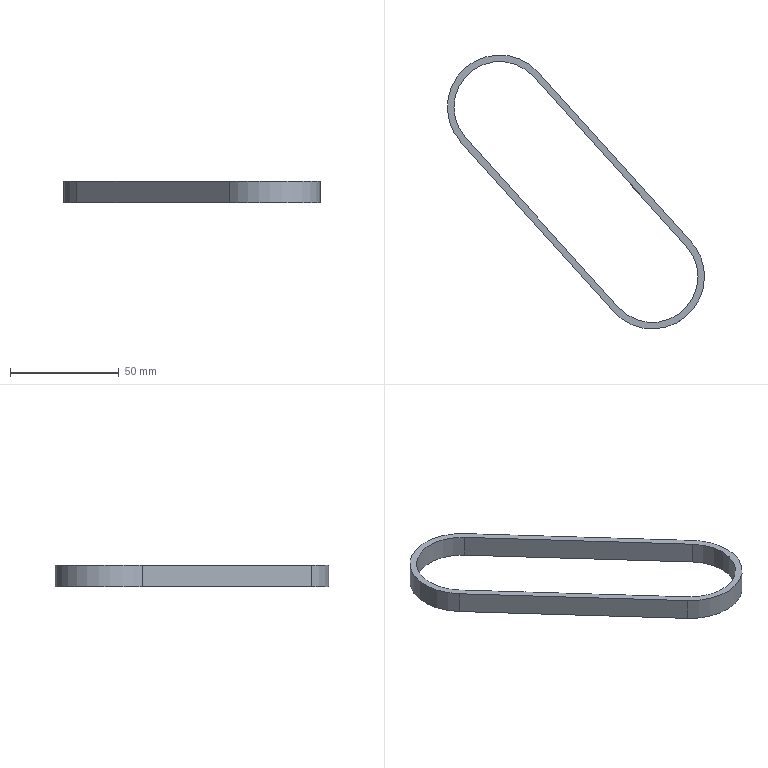Part | STEP file | 1 solid | 12 faces | box 118.296 x 125.997 x 10 mm | volume 10541 mm3 | plane 6 | cylinder 6 | commonest cylinder face diameters 42 x3 48 x3
STEP:
#1=CARTESIAN_POINT('',(0.,0.,0.));
#2=DIRECTION('',(0.,0.,1.));
#3=DIRECTION('',(1.,0.,0.));
#4=AXIS2_PLACEMENT_3D('',#1,#2,#3);
#5=CARTESIAN_POINT('',(15.599,14.059,-2.));
#6=VERTEX_POINT('',#5);
#7=CARTESIAN_POINT('',(-54.696,92.056,-2.));
#8=VERTEX_POINT('',#7);
#9=CARTESIAN_POINT('',(15.599,14.059,-2.));
#10=DIRECTION('',(-0.6695,0.7428,0.));
#11=VECTOR('',#10,1.);
#12=LINE('',#9,#11);
#13=CARTESIAN_POINT('',(15.599,14.059,-12.));
#14=DIRECTION('',(0.7428,0.6695,0.));
#15=DIRECTION('',(0.,0.,-1.));
#16=AXIS2_PLACEMENT_3D('',#13,#14,#15);
#17=PLANE('',#16);
#18=CARTESIAN_POINT('',(-10.,0.));
#19=DIRECTION('',(0.,1.));
#20=VECTOR('',#19,1.);
#21=LINE('',#18,#20);
#22=(GEOMETRIC_REPRESENTATION_CONTEXT(2)PARAMETRIC_REPRESENTATION_CONTEXT()REPRESENTATION_CONTEXT('',''));
#23=DEFINITIONAL_REPRESENTATION('',(#21),#22);
#24=PCURVE('',#17,#23);
#25=CARTESIAN_POINT('',(0.,0.,-2.));
#26=DIRECTION('',(0.,0.,1.));
#27=DIRECTION('',(0.,-1.,0.));
#28=AXIS2_PLACEMENT_3D('',#25,#26,#27);
#29=PLANE('',#28);
#30=CARTESIAN_POINT('',(-14.059,15.599));
#31=DIRECTION('',(-0.7428,-0.6695));
#32=VECTOR('',#31,1.);
#33=LINE('',#30,#32);
#34=(GEOMETRIC_REPRESENTATION_CONTEXT(2)PARAMETRIC_REPRESENTATION_CONTEXT()REPRESENTATION_CONTEXT('',''));
#35=DEFINITIONAL_REPRESENTATION('',(#33),#34);
#36=PCURVE('',#29,#35);
#37=SURFACE_CURVE('',#12,(#24,#36),.PCURVE_S1.);
#38=EDGE_CURVE('',#6,#8,#37,.T.);
#39=ORIENTED_EDGE('',*,*,#38,.T.);
#40=CARTESIAN_POINT('',(-54.696,92.056,-12.));
#41=VERTEX_POINT('',#40);
#42=CARTESIAN_POINT('',(-54.696,92.056,-12.));
#43=DIRECTION('',(0.,0.,1.));
#44=VECTOR('',#43,1.);
#45=LINE('',#42,#44);
#46=CARTESIAN_POINT('',(0.,105.));
#47=DIRECTION('',(-1.,0.));
#48=VECTOR('',#47,1.);
#49=LINE('',#46,#48);
#50=(GEOMETRIC_REPRESENTATION_CONTEXT(2)PARAMETRIC_REPRESENTATION_CONTEXT()REPRESENTATION_CONTEXT('',''));
#51=DEFINITIONAL_REPRESENTATION('',(#49),#50);
#52=PCURVE('',#17,#51);
#53=CARTESIAN_POINT('',(-70.296,77.997,-12.));
#54=DIRECTION('',(0.,0.,1.));
#55=DIRECTION('',(1.,0.,0.));
#56=AXIS2_PLACEMENT_3D('',#53,#54,#55);
#57=CYLINDRICAL_SURFACE('',#56,21.);
#58=CARTESIAN_POINT('',(0.7335,0.));
#59=DIRECTION('',(0.,1.));
#60=VECTOR('',#59,1.);
#61=LINE('',#58,#60);
#62=(GEOMETRIC_REPRESENTATION_CONTEXT(2)PARAMETRIC_REPRESENTATION_CONTEXT()REPRESENTATION_CONTEXT('',''));
#63=DEFINITIONAL_REPRESENTATION('',(#61),#62);
#64=PCURVE('',#57,#63);
#65=SURFACE_CURVE('',#45,(#52,#64),.PCURVE_S1.);
#66=EDGE_CURVE('',#41,#8,#65,.T.);
#67=ORIENTED_EDGE('',*,*,#66,.F.);
#68=CARTESIAN_POINT('',(15.599,14.059,-12.));
#69=VERTEX_POINT('',#68);
#70=CARTESIAN_POINT('',(15.599,14.059,-12.));
#71=DIRECTION('',(-0.6695,0.7428,0.));
#72=VECTOR('',#71,1.);
#73=LINE('',#70,#72);
#74=CARTESIAN_POINT('',(0.,0.));
#75=DIRECTION('',(0.,1.));
#76=VECTOR('',#75,1.);
#77=LINE('',#74,#76);
#78=(GEOMETRIC_REPRESENTATION_CONTEXT(2)PARAMETRIC_REPRESENTATION_CONTEXT()REPRESENTATION_CONTEXT('',''));
#79=DEFINITIONAL_REPRESENTATION('',(#77),#78);
#80=PCURVE('',#17,#79);
#81=CARTESIAN_POINT('',(0.,0.,-12.));
#82=DIRECTION('',(0.,0.,1.));
#83=DIRECTION('',(0.,-1.,0.));
#84=AXIS2_PLACEMENT_3D('',#81,#82,#83);
#85=PLANE('',#84);
#86=CARTESIAN_POINT('',(-14.059,15.599));
#87=DIRECTION('',(-0.7428,-0.6695));
#88=VECTOR('',#87,1.);
#89=LINE('',#86,#88);
#90=(GEOMETRIC_REPRESENTATION_CONTEXT(2)PARAMETRIC_REPRESENTATION_CONTEXT()REPRESENTATION_CONTEXT('',''));
#91=DEFINITIONAL_REPRESENTATION('',(#89),#90);
#92=PCURVE('',#85,#91);
#93=SURFACE_CURVE('',#73,(#80,#92),.PCURVE_S1.);
#94=EDGE_CURVE('',#69,#41,#93,.T.);
#95=ORIENTED_EDGE('',*,*,#94,.F.);
#96=CARTESIAN_POINT('',(15.599,14.059,-12.));
#97=DIRECTION('',(0.,0.,1.));
#98=VECTOR('',#97,1.);
#99=LINE('',#96,#98);
#100=CARTESIAN_POINT('',(0.,0.));
#101=DIRECTION('',(-1.,0.));
#102=VECTOR('',#101,1.);
#103=LINE('',#100,#102);
#104=(GEOMETRIC_REPRESENTATION_CONTEXT(2)PARAMETRIC_REPRESENTATION_CONTEXT()REPRESENTATION_CONTEXT('',''));
#105=DEFINITIONAL_REPRESENTATION('',(#103),#104);
#106=PCURVE('',#17,#105);
#107=CARTESIAN_POINT('',(0.,0.,-12.));
#108=DIRECTION('',(0.,0.,1.));
#109=DIRECTION('',(1.,0.,0.));
#110=AXIS2_PLACEMENT_3D('',#107,#108,#109);
#111=CYLINDRICAL_SURFACE('',#110,21.);
#112=CARTESIAN_POINT('',(0.7335,0.));
#113=DIRECTION('',(0.,1.));
#114=VECTOR('',#113,1.);
#115=LINE('',#112,#114);
#116=(GEOMETRIC_REPRESENTATION_CONTEXT(2)PARAMETRIC_REPRESENTATION_CONTEXT()REPRESENTATION_CONTEXT('',''));
#117=DEFINITIONAL_REPRESENTATION('',(#115),#116);
#118=PCURVE('',#111,#117);
#119=SURFACE_CURVE('',#99,(#106,#118),.PCURVE_S1.);
#120=EDGE_CURVE('',#69,#6,#119,.T.);
#121=ORIENTED_EDGE('',*,*,#120,.T.);
#122=EDGE_LOOP('',(#39,#67,#95,#121));
#123=FACE_BOUND('',#122,.T.);
#124=ADVANCED_FACE('',(#123),#17,.F.);
#125=ORIENTED_EDGE('',*,*,#66,.F.);
#126=CARTESIAN_POINT('',(-85.895,63.938,-12.));
#127=VERTEX_POINT('',#126);
#128=CARTESIAN_POINT('',(-70.296,77.997,-12.));
#129=DIRECTION('',(0.,0.,1.));
#130=DIRECTION('',(1.,0.,0.));
#131=AXIS2_PLACEMENT_3D('',#128,#129,#130);
#132=CIRCLE('',#131,21.);
#133=CARTESIAN_POINT('',(0.,0.));
#134=DIRECTION('',(1.,0.));
#135=VECTOR('',#134,1.);
#136=LINE('',#133,#135);
#137=(GEOMETRIC_REPRESENTATION_CONTEXT(2)PARAMETRIC_REPRESENTATION_CONTEXT()REPRESENTATION_CONTEXT('',''));
#138=DEFINITIONAL_REPRESENTATION('',(#136),#137);
#139=PCURVE('',#57,#138);
#140=CARTESIAN_POINT('',(-77.997,-70.296));
#141=DIRECTION('',(0.,1.));
#142=AXIS2_PLACEMENT_2D('',#140,#141);
#143=CIRCLE('',#142,21.);
#144=(GEOMETRIC_REPRESENTATION_CONTEXT(2)PARAMETRIC_REPRESENTATION_CONTEXT()REPRESENTATION_CONTEXT('',''));
#145=DEFINITIONAL_REPRESENTATION('',(#143),#144);
#146=PCURVE('',#85,#145);
#147=SURFACE_CURVE('',#132,(#139,#146),.PCURVE_S1.);
#148=EDGE_CURVE('',#41,#127,#147,.T.);
#149=ORIENTED_EDGE('',*,*,#148,.T.);
#150=CARTESIAN_POINT('',(-85.895,63.938,-2.));
#151=VERTEX_POINT('',#150);
#152=CARTESIAN_POINT('',(-85.895,63.938,-12.));
#153=DIRECTION('',(0.,0.,1.));
#154=VECTOR('',#153,1.);
#155=LINE('',#152,#154);
#156=CARTESIAN_POINT('',(3.875,0.));
#157=DIRECTION('',(0.,1.));
#158=VECTOR('',#157,1.);
#159=LINE('',#156,#158);
#160=(GEOMETRIC_REPRESENTATION_CONTEXT(2)PARAMETRIC_REPRESENTATION_CONTEXT()REPRESENTATION_CONTEXT('',''));
#161=DEFINITIONAL_REPRESENTATION('',(#159),#160);
#162=PCURVE('',#57,#161);
#163=CARTESIAN_POINT('',(-15.599,-14.059,-12.));
#164=DIRECTION('',(-0.7428,-0.6695,0.));
#165=DIRECTION('',(-0.6695,0.7428,0.));
#166=AXIS2_PLACEMENT_3D('',#163,#164,#165);
#167=PLANE('',#166);
#168=CARTESIAN_POINT('',(105.,0.));
#169=DIRECTION('',(0.,-1.));
#170=VECTOR('',#169,1.);
#171=LINE('',#168,#170);
#172=(GEOMETRIC_REPRESENTATION_CONTEXT(2)PARAMETRIC_REPRESENTATION_CONTEXT()REPRESENTATION_CONTEXT('',''));
#173=DEFINITIONAL_REPRESENTATION('',(#171),#172);
#174=PCURVE('',#167,#173);
#175=SURFACE_CURVE('',#155,(#162,#174),.PCURVE_S1.);
#176=EDGE_CURVE('',#127,#151,#175,.T.);
#177=ORIENTED_EDGE('',*,*,#176,.T.);
#178=CARTESIAN_POINT('',(-70.296,77.997,-2.));
#179=DIRECTION('',(0.,0.,1.));
#180=DIRECTION('',(1.,0.,0.));
#181=AXIS2_PLACEMENT_3D('',#178,#179,#180);
#182=CIRCLE('',#181,21.);
#183=CARTESIAN_POINT('',(0.,10.));
#184=DIRECTION('',(1.,0.));
#185=VECTOR('',#184,1.);
#186=LINE('',#183,#185);
#187=(GEOMETRIC_REPRESENTATION_CONTEXT(2)PARAMETRIC_REPRESENTATION_CONTEXT()REPRESENTATION_CONTEXT('',''));
#188=DEFINITIONAL_REPRESENTATION('',(#186),#187);
#189=PCURVE('',#57,#188);
#190=CARTESIAN_POINT('',(-77.997,-70.296));
#191=DIRECTION('',(0.,1.));
#192=AXIS2_PLACEMENT_2D('',#190,#191);
#193=CIRCLE('',#192,21.);
#194=(GEOMETRIC_REPRESENTATION_CONTEXT(2)PARAMETRIC_REPRESENTATION_CONTEXT()REPRESENTATION_CONTEXT('',''));
#195=DEFINITIONAL_REPRESENTATION('',(#193),#194);
#196=PCURVE('',#29,#195);
#197=SURFACE_CURVE('',#182,(#189,#196),.PCURVE_S1.);
#198=EDGE_CURVE('',#8,#151,#197,.T.);
#199=ORIENTED_EDGE('',*,*,#198,.F.);
#200=EDGE_LOOP('',(#125,#149,#177,#199));
#201=FACE_BOUND('',#200,.F.);
#202=ADVANCED_FACE('',(#201),#57,.F.);
#203=CARTESIAN_POINT('',(-15.599,-14.059,-2.));
#204=VERTEX_POINT('',#203);
#205=CARTESIAN_POINT('',(-15.599,-14.059,-2.));
#206=DIRECTION('',(0.6695,-0.7428,0.));
#207=VECTOR('',#206,1.);
#208=LINE('',#205,#207);
#209=CARTESIAN_POINT('',(0.,-10.));
#210=DIRECTION('',(-1.,0.));
#211=VECTOR('',#210,1.);
#212=LINE('',#209,#211);
#213=(GEOMETRIC_REPRESENTATION_CONTEXT(2)PARAMETRIC_REPRESENTATION_CONTEXT()REPRESENTATION_CONTEXT('',''));
#214=DEFINITIONAL_REPRESENTATION('',(#212),#213);
#215=PCURVE('',#167,#214);
#216=CARTESIAN_POINT('',(14.059,-15.599));
#217=DIRECTION('',(0.7428,0.6695));
#218=VECTOR('',#217,1.);
#219=LINE('',#216,#218);
#220=(GEOMETRIC_REPRESENTATION_CONTEXT(2)PARAMETRIC_REPRESENTATION_CONTEXT()REPRESENTATION_CONTEXT('',''));
#221=DEFINITIONAL_REPRESENTATION('',(#219),#220);
#222=PCURVE('',#29,#221);
#223=SURFACE_CURVE('',#208,(#215,#222),.PCURVE_S1.);
#224=EDGE_CURVE('',#151,#204,#223,.T.);
#225=ORIENTED_EDGE('',*,*,#224,.T.);
#226=CARTESIAN_POINT('',(-15.599,-14.059,-12.));
#227=VERTEX_POINT('',#226);
#228=CARTESIAN_POINT('',(-15.599,-14.059,-12.));
#229=DIRECTION('',(0.,0.,1.));
#230=VECTOR('',#229,1.);
#231=LINE('',#228,#230);
#232=CARTESIAN_POINT('',(0.,0.));
#233=DIRECTION('',(0.,-1.));
#234=VECTOR('',#233,1.);
#235=LINE('',#232,#234);
#236=(GEOMETRIC_REPRESENTATION_CONTEXT(2)PARAMETRIC_REPRESENTATION_CONTEXT()REPRESENTATION_CONTEXT('',''));
#237=DEFINITIONAL_REPRESENTATION('',(#235),#236);
#238=PCURVE('',#167,#237);
#239=CARTESIAN_POINT('',(0.,0.,-12.));
#240=DIRECTION('',(0.,0.,1.));
#241=DIRECTION('',(1.,0.,0.));
#242=AXIS2_PLACEMENT_3D('',#239,#240,#241);
#243=CYLINDRICAL_SURFACE('',#242,21.);
#244=CARTESIAN_POINT('',(3.875,0.));
#245=DIRECTION('',(0.,1.));
#246=VECTOR('',#245,1.);
#247=LINE('',#244,#246);
#248=(GEOMETRIC_REPRESENTATION_CONTEXT(2)PARAMETRIC_REPRESENTATION_CONTEXT()REPRESENTATION_CONTEXT('',''));
#249=DEFINITIONAL_REPRESENTATION('',(#247),#248);
#250=PCURVE('',#243,#249);
#251=SURFACE_CURVE('',#231,(#238,#250),.PCURVE_S1.);
#252=EDGE_CURVE('',#227,#204,#251,.T.);
#253=ORIENTED_EDGE('',*,*,#252,.F.);
#254=CARTESIAN_POINT('',(-15.599,-14.059,-12.));
#255=DIRECTION('',(0.6695,-0.7428,0.));
#256=VECTOR('',#255,1.);
#257=LINE('',#254,#256);
#258=CARTESIAN_POINT('',(0.,0.));
#259=DIRECTION('',(-1.,0.));
#260=VECTOR('',#259,1.);
#261=LINE('',#258,#260);
#262=(GEOMETRIC_REPRESENTATION_CONTEXT(2)PARAMETRIC_REPRESENTATION_CONTEXT()REPRESENTATION_CONTEXT('',''));
#263=DEFINITIONAL_REPRESENTATION('',(#261),#262);
#264=PCURVE('',#167,#263);
#265=CARTESIAN_POINT('',(14.059,-15.599));
#266=DIRECTION('',(0.7428,0.6695));
#267=VECTOR('',#266,1.);
#268=LINE('',#265,#267);
#269=(GEOMETRIC_REPRESENTATION_CONTEXT(2)PARAMETRIC_REPRESENTATION_CONTEXT()REPRESENTATION_CONTEXT('',''));
#270=DEFINITIONAL_REPRESENTATION('',(#268),#269);
#271=PCURVE('',#85,#270);
#272=SURFACE_CURVE('',#257,(#264,#271),.PCURVE_S1.);
#273=EDGE_CURVE('',#127,#227,#272,.T.);
#274=ORIENTED_EDGE('',*,*,#273,.F.);
#275=ORIENTED_EDGE('',*,*,#176,.T.);
#276=EDGE_LOOP('',(#225,#253,#274,#275));
#277=FACE_BOUND('',#276,.T.);
#278=ADVANCED_FACE('',(#277),#167,.F.);
#279=CARTESIAN_POINT('',(21.,0.,-2.));
#280=VERTEX_POINT('',#279);
#281=CARTESIAN_POINT('',(0.,0.,-2.));
#282=DIRECTION('',(0.,0.,1.));
#283=DIRECTION('',(1.,0.,0.));
#284=AXIS2_PLACEMENT_3D('',#281,#282,#283);
#285=CIRCLE('',#284,21.);
#286=CARTESIAN_POINT('',(0.,10.));
#287=DIRECTION('',(1.,0.));
#288=VECTOR('',#287,1.);
#289=LINE('',#286,#288);
#290=(GEOMETRIC_REPRESENTATION_CONTEXT(2)PARAMETRIC_REPRESENTATION_CONTEXT()REPRESENTATION_CONTEXT('',''));
#291=DEFINITIONAL_REPRESENTATION('',(#289),#290);
#292=PCURVE('',#243,#291);
#293=CARTESIAN_POINT('',(0.,0.));
#294=DIRECTION('',(0.,1.));
#295=AXIS2_PLACEMENT_2D('',#293,#294);
#296=CIRCLE('',#295,21.);
#297=(GEOMETRIC_REPRESENTATION_CONTEXT(2)PARAMETRIC_REPRESENTATION_CONTEXT()REPRESENTATION_CONTEXT('',''));
#298=DEFINITIONAL_REPRESENTATION('',(#296),#297);
#299=PCURVE('',#29,#298);
#300=SURFACE_CURVE('',#285,(#292,#299),.PCURVE_S1.);
#301=EDGE_CURVE('',#204,#280,#300,.T.);
#302=ORIENTED_EDGE('',*,*,#301,.F.);
#303=ORIENTED_EDGE('',*,*,#252,.F.);
#304=CARTESIAN_POINT('',(21.,0.,-12.));
#305=VERTEX_POINT('',#304);
#306=CARTESIAN_POINT('',(0.,0.,-12.));
#307=DIRECTION('',(0.,0.,1.));
#308=DIRECTION('',(1.,0.,0.));
#309=AXIS2_PLACEMENT_3D('',#306,#307,#308);
#310=CIRCLE('',#309,21.);
#311=CARTESIAN_POINT('',(0.,0.));
#312=DIRECTION('',(1.,0.));
#313=VECTOR('',#312,1.);
#314=LINE('',#311,#313);
#315=(GEOMETRIC_REPRESENTATION_CONTEXT(2)PARAMETRIC_REPRESENTATION_CONTEXT()REPRESENTATION_CONTEXT('',''));
#316=DEFINITIONAL_REPRESENTATION('',(#314),#315);
#317=PCURVE('',#243,#316);
#318=CARTESIAN_POINT('',(0.,0.));
#319=DIRECTION('',(0.,1.));
#320=AXIS2_PLACEMENT_2D('',#318,#319);
#321=CIRCLE('',#320,21.);
#322=(GEOMETRIC_REPRESENTATION_CONTEXT(2)PARAMETRIC_REPRESENTATION_CONTEXT()REPRESENTATION_CONTEXT('',''));
#323=DEFINITIONAL_REPRESENTATION('',(#321),#322);
#324=PCURVE('',#85,#323);
#325=SURFACE_CURVE('',#310,(#317,#324),.PCURVE_S1.);
#326=EDGE_CURVE('',#227,#305,#325,.T.);
#327=ORIENTED_EDGE('',*,*,#326,.T.);
#328=CARTESIAN_POINT('',(21.,0.,-12.));
#329=DIRECTION('',(0.,0.,1.));
#330=VECTOR('',#329,1.);
#331=LINE('',#328,#330);
#332=CARTESIAN_POINT('',(6.283,0.));
#333=DIRECTION('',(0.,1.));
#334=VECTOR('',#333,1.);
#335=LINE('',#332,#334);
#336=(GEOMETRIC_REPRESENTATION_CONTEXT(2)PARAMETRIC_REPRESENTATION_CONTEXT()REPRESENTATION_CONTEXT('',''));
#337=DEFINITIONAL_REPRESENTATION('',(#335),#336);
#338=PCURVE('',#243,#337);
#339=CARTESIAN_POINT('',(0.,0.));
#340=DIRECTION('',(0.,1.));
#341=VECTOR('',#340,1.);
#342=LINE('',#339,#341);
#343=(GEOMETRIC_REPRESENTATION_CONTEXT(2)PARAMETRIC_REPRESENTATION_CONTEXT()REPRESENTATION_CONTEXT('',''));
#344=DEFINITIONAL_REPRESENTATION('',(#342),#343);
#345=PCURVE('',#111,#344);
#346=SURFACE_CURVE('',#331,(#338,#345),.PCURVE_S1.);
#347=EDGE_CURVE('',#305,#280,#346,.T.);
#348=ORIENTED_EDGE('',*,*,#347,.T.);
#349=EDGE_LOOP('',(#302,#303,#327,#348));
#350=FACE_BOUND('',#349,.F.);
#351=ADVANCED_FACE('',(#350),#243,.F.);
#352=ORIENTED_EDGE('',*,*,#301,.F.);
#353=ORIENTED_EDGE('',*,*,#224,.F.);
#354=ORIENTED_EDGE('',*,*,#198,.F.);
#355=ORIENTED_EDGE('',*,*,#38,.F.);
#356=CARTESIAN_POINT('',(0.,0.,-2.));
#357=DIRECTION('',(0.,0.,1.));
#358=DIRECTION('',(1.,0.,0.));
#359=AXIS2_PLACEMENT_3D('',#356,#357,#358);
#360=CIRCLE('',#359,21.);
#361=CARTESIAN_POINT('',(0.,0.));
#362=DIRECTION('',(0.,1.));
#363=AXIS2_PLACEMENT_2D('',#361,#362);
#364=CIRCLE('',#363,21.);
#365=(GEOMETRIC_REPRESENTATION_CONTEXT(2)PARAMETRIC_REPRESENTATION_CONTEXT()REPRESENTATION_CONTEXT('',''));
#366=DEFINITIONAL_REPRESENTATION('',(#364),#365);
#367=PCURVE('',#29,#366);
#368=CARTESIAN_POINT('',(0.,10.));
#369=DIRECTION('',(1.,0.));
#370=VECTOR('',#369,1.);
#371=LINE('',#368,#370);
#372=(GEOMETRIC_REPRESENTATION_CONTEXT(2)PARAMETRIC_REPRESENTATION_CONTEXT()REPRESENTATION_CONTEXT('',''));
#373=DEFINITIONAL_REPRESENTATION('',(#371),#372);
#374=PCURVE('',#111,#373);
#375=SURFACE_CURVE('',#360,(#367,#374),.PCURVE_S1.);
#376=EDGE_CURVE('',#280,#6,#375,.T.);
#377=ORIENTED_EDGE('',*,*,#376,.F.);
#378=EDGE_LOOP('',(#352,#353,#354,#355,#377));
#379=FACE_BOUND('',#378,.T.);
#380=CARTESIAN_POINT('',(-17.828,-16.068,-2.));
#381=VERTEX_POINT('',#380);
#382=CARTESIAN_POINT('',(24.,0.,-2.));
#383=VERTEX_POINT('',#382);
#384=CARTESIAN_POINT('',(0.,0.,-2.));
#385=DIRECTION('',(0.,0.,1.));
#386=DIRECTION('',(1.,0.,0.));
#387=AXIS2_PLACEMENT_3D('',#384,#385,#386);
#388=CIRCLE('',#387,24.);
#389=CARTESIAN_POINT('',(0.,0.));
#390=DIRECTION('',(0.,1.));
#391=AXIS2_PLACEMENT_2D('',#389,#390);
#392=CIRCLE('',#391,24.);
#393=(GEOMETRIC_REPRESENTATION_CONTEXT(2)PARAMETRIC_REPRESENTATION_CONTEXT()REPRESENTATION_CONTEXT('',''));
#394=DEFINITIONAL_REPRESENTATION('',(#392),#393);
#395=PCURVE('',#29,#394);
#396=CARTESIAN_POINT('',(0.,0.,-12.));
#397=DIRECTION('',(0.,0.,1.));
#398=DIRECTION('',(1.,0.,0.));
#399=AXIS2_PLACEMENT_3D('',#396,#397,#398);
#400=CYLINDRICAL_SURFACE('',#399,24.);
#401=CARTESIAN_POINT('',(0.,10.));
#402=DIRECTION('',(1.,0.));
#403=VECTOR('',#402,1.);
#404=LINE('',#401,#403);
#405=(GEOMETRIC_REPRESENTATION_CONTEXT(2)PARAMETRIC_REPRESENTATION_CONTEXT()REPRESENTATION_CONTEXT('',''));
#406=DEFINITIONAL_REPRESENTATION('',(#404),#405);
#407=PCURVE('',#400,#406);
#408=SURFACE_CURVE('',#388,(#395,#407),.PCURVE_S1.);
#409=EDGE_CURVE('',#381,#383,#408,.T.);
#410=ORIENTED_EDGE('',*,*,#409,.T.);
#411=CARTESIAN_POINT('',(17.828,16.068,-2.));
#412=VERTEX_POINT('',#411);
#413=CARTESIAN_POINT('',(0.,0.,-2.));
#414=DIRECTION('',(0.,0.,1.));
#415=DIRECTION('',(1.,0.,0.));
#416=AXIS2_PLACEMENT_3D('',#413,#414,#415);
#417=CIRCLE('',#416,24.);
#418=CARTESIAN_POINT('',(0.,0.));
#419=DIRECTION('',(0.,1.));
#420=AXIS2_PLACEMENT_2D('',#418,#419);
#421=CIRCLE('',#420,24.);
#422=(GEOMETRIC_REPRESENTATION_CONTEXT(2)PARAMETRIC_REPRESENTATION_CONTEXT()REPRESENTATION_CONTEXT('',''));
#423=DEFINITIONAL_REPRESENTATION('',(#421),#422);
#424=PCURVE('',#29,#423);
#425=CARTESIAN_POINT('',(0.,0.,-12.));
#426=DIRECTION('',(0.,0.,1.));
#427=DIRECTION('',(1.,0.,0.));
#428=AXIS2_PLACEMENT_3D('',#425,#426,#427);
#429=CYLINDRICAL_SURFACE('',#428,24.);
#430=CARTESIAN_POINT('',(0.,10.));
#431=DIRECTION('',(1.,0.));
#432=VECTOR('',#431,1.);
#433=LINE('',#430,#432);
#434=(GEOMETRIC_REPRESENTATION_CONTEXT(2)PARAMETRIC_REPRESENTATION_CONTEXT()REPRESENTATION_CONTEXT('',''));
#435=DEFINITIONAL_REPRESENTATION('',(#433),#434);
#436=PCURVE('',#429,#435);
#437=SURFACE_CURVE('',#417,(#424,#436),.PCURVE_S1.);
#438=EDGE_CURVE('',#383,#412,#437,.T.);
#439=ORIENTED_EDGE('',*,*,#438,.T.);
#440=CARTESIAN_POINT('',(-52.468,94.064,-2.));
#441=VERTEX_POINT('',#440);
#442=CARTESIAN_POINT('',(17.828,16.068,-2.));
#443=DIRECTION('',(-0.6695,0.7428,0.));
#444=VECTOR('',#443,1.);
#445=LINE('',#442,#444);
#446=CARTESIAN_POINT('',(-16.068,17.828));
#447=DIRECTION('',(-0.7428,-0.6695));
#448=VECTOR('',#447,1.);
#449=LINE('',#446,#448);
#450=(GEOMETRIC_REPRESENTATION_CONTEXT(2)PARAMETRIC_REPRESENTATION_CONTEXT()REPRESENTATION_CONTEXT('',''));
#451=DEFINITIONAL_REPRESENTATION('',(#449),#450);
#452=PCURVE('',#29,#451);
#453=CARTESIAN_POINT('',(17.828,16.068,-12.));
#454=DIRECTION('',(0.7428,0.6695,0.));
#455=DIRECTION('',(0.,0.,-1.));
#456=AXIS2_PLACEMENT_3D('',#453,#454,#455);
#457=PLANE('',#456);
#458=CARTESIAN_POINT('',(-10.,0.));
#459=DIRECTION('',(0.,1.));
#460=VECTOR('',#459,1.);
#461=LINE('',#458,#460);
#462=(GEOMETRIC_REPRESENTATION_CONTEXT(2)PARAMETRIC_REPRESENTATION_CONTEXT()REPRESENTATION_CONTEXT('',''));
#463=DEFINITIONAL_REPRESENTATION('',(#461),#462);
#464=PCURVE('',#457,#463);
#465=SURFACE_CURVE('',#445,(#452,#464),.PCURVE_S1.);
#466=EDGE_CURVE('',#412,#441,#465,.T.);
#467=ORIENTED_EDGE('',*,*,#466,.T.);
#468=CARTESIAN_POINT('',(-88.124,61.929,-2.));
#469=VERTEX_POINT('',#468);
#470=CARTESIAN_POINT('',(-70.296,77.997,-2.));
#471=DIRECTION('',(0.,0.,1.));
#472=DIRECTION('',(1.,0.,0.));
#473=AXIS2_PLACEMENT_3D('',#470,#471,#472);
#474=CIRCLE('',#473,24.);
#475=CARTESIAN_POINT('',(-77.997,-70.296));
#476=DIRECTION('',(0.,1.));
#477=AXIS2_PLACEMENT_2D('',#475,#476);
#478=CIRCLE('',#477,24.);
#479=(GEOMETRIC_REPRESENTATION_CONTEXT(2)PARAMETRIC_REPRESENTATION_CONTEXT()REPRESENTATION_CONTEXT('',''));
#480=DEFINITIONAL_REPRESENTATION('',(#478),#479);
#481=PCURVE('',#29,#480);
#482=CARTESIAN_POINT('',(-70.296,77.997,-12.));
#483=DIRECTION('',(0.,0.,1.));
#484=DIRECTION('',(1.,0.,0.));
#485=AXIS2_PLACEMENT_3D('',#482,#483,#484);
#486=CYLINDRICAL_SURFACE('',#485,24.);
#487=CARTESIAN_POINT('',(0.,10.));
#488=DIRECTION('',(1.,0.));
#489=VECTOR('',#488,1.);
#490=LINE('',#487,#489);
#491=(GEOMETRIC_REPRESENTATION_CONTEXT(2)PARAMETRIC_REPRESENTATION_CONTEXT()REPRESENTATION_CONTEXT('',''));
#492=DEFINITIONAL_REPRESENTATION('',(#490),#491);
#493=PCURVE('',#486,#492);
#494=SURFACE_CURVE('',#474,(#481,#493),.PCURVE_S1.);
#495=EDGE_CURVE('',#441,#469,#494,.T.);
#496=ORIENTED_EDGE('',*,*,#495,.T.);
#497=CARTESIAN_POINT('',(-17.828,-16.068,-2.));
#498=DIRECTION('',(0.6695,-0.7428,0.));
#499=VECTOR('',#498,1.);
#500=LINE('',#497,#499);
#501=CARTESIAN_POINT('',(16.068,-17.828));
#502=DIRECTION('',(0.7428,0.6695));
#503=VECTOR('',#502,1.);
#504=LINE('',#501,#503);
#505=(GEOMETRIC_REPRESENTATION_CONTEXT(2)PARAMETRIC_REPRESENTATION_CONTEXT()REPRESENTATION_CONTEXT('',''));
#506=DEFINITIONAL_REPRESENTATION('',(#504),#505);
#507=PCURVE('',#29,#506);
#508=CARTESIAN_POINT('',(-17.828,-16.068,-12.));
#509=DIRECTION('',(-0.7428,-0.6695,0.));
#510=DIRECTION('',(-0.6695,0.7428,0.));
#511=AXIS2_PLACEMENT_3D('',#508,#509,#510);
#512=PLANE('',#511);
#513=CARTESIAN_POINT('',(0.,-10.));
#514=DIRECTION('',(-1.,0.));
#515=VECTOR('',#514,1.);
#516=LINE('',#513,#515);
#517=(GEOMETRIC_REPRESENTATION_CONTEXT(2)PARAMETRIC_REPRESENTATION_CONTEXT()REPRESENTATION_CONTEXT('',''));
#518=DEFINITIONAL_REPRESENTATION('',(#516),#517);
#519=PCURVE('',#512,#518);
#520=SURFACE_CURVE('',#500,(#507,#519),.PCURVE_S1.);
#521=EDGE_CURVE('',#469,#381,#520,.T.);
#522=ORIENTED_EDGE('',*,*,#521,.T.);
#523=EDGE_LOOP('',(#410,#439,#467,#496,#522));
#524=FACE_BOUND('',#523,.T.);
#525=ADVANCED_FACE('',(#379,#524),#29,.T.);
#526=ORIENTED_EDGE('',*,*,#273,.T.);
#527=ORIENTED_EDGE('',*,*,#326,.T.);
#528=CARTESIAN_POINT('',(0.,0.,-12.));
#529=DIRECTION('',(0.,0.,1.));
#530=DIRECTION('',(1.,0.,0.));
#531=AXIS2_PLACEMENT_3D('',#528,#529,#530);
#532=CIRCLE('',#531,21.);
#533=CARTESIAN_POINT('',(0.,0.));
#534=DIRECTION('',(0.,1.));
#535=AXIS2_PLACEMENT_2D('',#533,#534);
#536=CIRCLE('',#535,21.);
#537=(GEOMETRIC_REPRESENTATION_CONTEXT(2)PARAMETRIC_REPRESENTATION_CONTEXT()REPRESENTATION_CONTEXT('',''));
#538=DEFINITIONAL_REPRESENTATION('',(#536),#537);
#539=PCURVE('',#85,#538);
#540=CARTESIAN_POINT('',(0.,0.));
#541=DIRECTION('',(1.,0.));
#542=VECTOR('',#541,1.);
#543=LINE('',#540,#542);
#544=(GEOMETRIC_REPRESENTATION_CONTEXT(2)PARAMETRIC_REPRESENTATION_CONTEXT()REPRESENTATION_CONTEXT('',''));
#545=DEFINITIONAL_REPRESENTATION('',(#543),#544);
#546=PCURVE('',#111,#545);
#547=SURFACE_CURVE('',#532,(#539,#546),.PCURVE_S1.);
#548=EDGE_CURVE('',#305,#69,#547,.T.);
#549=ORIENTED_EDGE('',*,*,#548,.T.);
#550=ORIENTED_EDGE('',*,*,#94,.T.);
#551=ORIENTED_EDGE('',*,*,#148,.T.);
#552=EDGE_LOOP('',(#526,#527,#549,#550,#551));
#553=FACE_BOUND('',#552,.T.);
#554=CARTESIAN_POINT('',(-17.828,-16.068,-12.));
#555=VERTEX_POINT('',#554);
#556=CARTESIAN_POINT('',(24.,0.,-12.));
#557=VERTEX_POINT('',#556);
#558=CARTESIAN_POINT('',(0.,0.,-12.));
#559=DIRECTION('',(0.,0.,1.));
#560=DIRECTION('',(1.,0.,0.));
#561=AXIS2_PLACEMENT_3D('',#558,#559,#560);
#562=CIRCLE('',#561,24.);
#563=CARTESIAN_POINT('',(0.,0.));
#564=DIRECTION('',(0.,1.));
#565=AXIS2_PLACEMENT_2D('',#563,#564);
#566=CIRCLE('',#565,24.);
#567=(GEOMETRIC_REPRESENTATION_CONTEXT(2)PARAMETRIC_REPRESENTATION_CONTEXT()REPRESENTATION_CONTEXT('',''));
#568=DEFINITIONAL_REPRESENTATION('',(#566),#567);
#569=PCURVE('',#85,#568);
#570=CARTESIAN_POINT('',(0.,0.));
#571=DIRECTION('',(1.,0.));
#572=VECTOR('',#571,1.);
#573=LINE('',#570,#572);
#574=(GEOMETRIC_REPRESENTATION_CONTEXT(2)PARAMETRIC_REPRESENTATION_CONTEXT()REPRESENTATION_CONTEXT('',''));
#575=DEFINITIONAL_REPRESENTATION('',(#573),#574);
#576=PCURVE('',#400,#575);
#577=SURFACE_CURVE('',#562,(#569,#576),.PCURVE_S1.);
#578=EDGE_CURVE('',#555,#557,#577,.T.);
#579=ORIENTED_EDGE('',*,*,#578,.F.);
#580=CARTESIAN_POINT('',(-88.124,61.929,-12.));
#581=VERTEX_POINT('',#580);
#582=CARTESIAN_POINT('',(-17.828,-16.068,-12.));
#583=DIRECTION('',(0.6695,-0.7428,0.));
#584=VECTOR('',#583,1.);
#585=LINE('',#582,#584);
#586=CARTESIAN_POINT('',(16.068,-17.828));
#587=DIRECTION('',(0.7428,0.6695));
#588=VECTOR('',#587,1.);
#589=LINE('',#586,#588);
#590=(GEOMETRIC_REPRESENTATION_CONTEXT(2)PARAMETRIC_REPRESENTATION_CONTEXT()REPRESENTATION_CONTEXT('',''));
#591=DEFINITIONAL_REPRESENTATION('',(#589),#590);
#592=PCURVE('',#85,#591);
#593=CARTESIAN_POINT('',(0.,0.));
#594=DIRECTION('',(-1.,0.));
#595=VECTOR('',#594,1.);
#596=LINE('',#593,#595);
#597=(GEOMETRIC_REPRESENTATION_CONTEXT(2)PARAMETRIC_REPRESENTATION_CONTEXT()REPRESENTATION_CONTEXT('',''));
#598=DEFINITIONAL_REPRESENTATION('',(#596),#597);
#599=PCURVE('',#512,#598);
#600=SURFACE_CURVE('',#585,(#592,#599),.PCURVE_S1.);
#601=EDGE_CURVE('',#581,#555,#600,.T.);
#602=ORIENTED_EDGE('',*,*,#601,.F.);
#603=CARTESIAN_POINT('',(-52.468,94.064,-12.));
#604=VERTEX_POINT('',#603);
#605=CARTESIAN_POINT('',(-70.296,77.997,-12.));
#606=DIRECTION('',(0.,0.,1.));
#607=DIRECTION('',(1.,0.,0.));
#608=AXIS2_PLACEMENT_3D('',#605,#606,#607);
#609=CIRCLE('',#608,24.);
#610=CARTESIAN_POINT('',(-77.997,-70.296));
#611=DIRECTION('',(0.,1.));
#612=AXIS2_PLACEMENT_2D('',#610,#611);
#613=CIRCLE('',#612,24.);
#614=(GEOMETRIC_REPRESENTATION_CONTEXT(2)PARAMETRIC_REPRESENTATION_CONTEXT()REPRESENTATION_CONTEXT('',''));
#615=DEFINITIONAL_REPRESENTATION('',(#613),#614);
#616=PCURVE('',#85,#615);
#617=CARTESIAN_POINT('',(0.,0.));
#618=DIRECTION('',(1.,0.));
#619=VECTOR('',#618,1.);
#620=LINE('',#617,#619);
#621=(GEOMETRIC_REPRESENTATION_CONTEXT(2)PARAMETRIC_REPRESENTATION_CONTEXT()REPRESENTATION_CONTEXT('',''));
#622=DEFINITIONAL_REPRESENTATION('',(#620),#621);
#623=PCURVE('',#486,#622);
#624=SURFACE_CURVE('',#609,(#616,#623),.PCURVE_S1.);
#625=EDGE_CURVE('',#604,#581,#624,.T.);
#626=ORIENTED_EDGE('',*,*,#625,.F.);
#627=CARTESIAN_POINT('',(17.828,16.068,-12.));
#628=VERTEX_POINT('',#627);
#629=CARTESIAN_POINT('',(17.828,16.068,-12.));
#630=DIRECTION('',(-0.6695,0.7428,0.));
#631=VECTOR('',#630,1.);
#632=LINE('',#629,#631);
#633=CARTESIAN_POINT('',(-16.068,17.828));
#634=DIRECTION('',(-0.7428,-0.6695));
#635=VECTOR('',#634,1.);
#636=LINE('',#633,#635);
#637=(GEOMETRIC_REPRESENTATION_CONTEXT(2)PARAMETRIC_REPRESENTATION_CONTEXT()REPRESENTATION_CONTEXT('',''));
#638=DEFINITIONAL_REPRESENTATION('',(#636),#637);
#639=PCURVE('',#85,#638);
#640=CARTESIAN_POINT('',(0.,0.));
#641=DIRECTION('',(0.,1.));
#642=VECTOR('',#641,1.);
#643=LINE('',#640,#642);
#644=(GEOMETRIC_REPRESENTATION_CONTEXT(2)PARAMETRIC_REPRESENTATION_CONTEXT()REPRESENTATION_CONTEXT('',''));
#645=DEFINITIONAL_REPRESENTATION('',(#643),#644);
#646=PCURVE('',#457,#645);
#647=SURFACE_CURVE('',#632,(#639,#646),.PCURVE_S1.);
#648=EDGE_CURVE('',#628,#604,#647,.T.);
#649=ORIENTED_EDGE('',*,*,#648,.F.);
#650=CARTESIAN_POINT('',(0.,0.,-12.));
#651=DIRECTION('',(0.,0.,1.));
#652=DIRECTION('',(1.,0.,0.));
#653=AXIS2_PLACEMENT_3D('',#650,#651,#652);
#654=CIRCLE('',#653,24.);
#655=CARTESIAN_POINT('',(0.,0.));
#656=DIRECTION('',(0.,1.));
#657=AXIS2_PLACEMENT_2D('',#655,#656);
#658=CIRCLE('',#657,24.);
#659=(GEOMETRIC_REPRESENTATION_CONTEXT(2)PARAMETRIC_REPRESENTATION_CONTEXT()REPRESENTATION_CONTEXT('',''));
#660=DEFINITIONAL_REPRESENTATION('',(#658),#659);
#661=PCURVE('',#85,#660);
#662=CARTESIAN_POINT('',(0.,0.));
#663=DIRECTION('',(1.,0.));
#664=VECTOR('',#663,1.);
#665=LINE('',#662,#664);
#666=(GEOMETRIC_REPRESENTATION_CONTEXT(2)PARAMETRIC_REPRESENTATION_CONTEXT()REPRESENTATION_CONTEXT('',''));
#667=DEFINITIONAL_REPRESENTATION('',(#665),#666);
#668=PCURVE('',#429,#667);
#669=SURFACE_CURVE('',#654,(#661,#668),.PCURVE_S1.);
#670=EDGE_CURVE('',#557,#628,#669,.T.);
#671=ORIENTED_EDGE('',*,*,#670,.F.);
#672=EDGE_LOOP('',(#579,#602,#626,#649,#671));
#673=FACE_BOUND('',#672,.T.);
#674=ADVANCED_FACE('',(#553,#673),#85,.F.);
#675=ORIENTED_EDGE('',*,*,#466,.F.);
#676=CARTESIAN_POINT('',(17.828,16.068,-12.));
#677=DIRECTION('',(0.,0.,1.));
#678=VECTOR('',#677,1.);
#679=LINE('',#676,#678);
#680=CARTESIAN_POINT('',(0.,0.));
#681=DIRECTION('',(-1.,0.));
#682=VECTOR('',#681,1.);
#683=LINE('',#680,#682);
#684=(GEOMETRIC_REPRESENTATION_CONTEXT(2)PARAMETRIC_REPRESENTATION_CONTEXT()REPRESENTATION_CONTEXT('',''));
#685=DEFINITIONAL_REPRESENTATION('',(#683),#684);
#686=PCURVE('',#457,#685);
#687=CARTESIAN_POINT('',(0.7335,0.));
#688=DIRECTION('',(0.,1.));
#689=VECTOR('',#688,1.);
#690=LINE('',#687,#689);
#691=(GEOMETRIC_REPRESENTATION_CONTEXT(2)PARAMETRIC_REPRESENTATION_CONTEXT()REPRESENTATION_CONTEXT('',''));
#692=DEFINITIONAL_REPRESENTATION('',(#690),#691);
#693=PCURVE('',#429,#692);
#694=SURFACE_CURVE('',#679,(#686,#693),.PCURVE_S1.);
#695=EDGE_CURVE('',#628,#412,#694,.T.);
#696=ORIENTED_EDGE('',*,*,#695,.F.);
#697=ORIENTED_EDGE('',*,*,#648,.T.);
#698=CARTESIAN_POINT('',(-52.468,94.064,-12.));
#699=DIRECTION('',(0.,0.,1.));
#700=VECTOR('',#699,1.);
#701=LINE('',#698,#700);
#702=CARTESIAN_POINT('',(0.,105.));
#703=DIRECTION('',(-1.,0.));
#704=VECTOR('',#703,1.);
#705=LINE('',#702,#704);
#706=(GEOMETRIC_REPRESENTATION_CONTEXT(2)PARAMETRIC_REPRESENTATION_CONTEXT()REPRESENTATION_CONTEXT('',''));
#707=DEFINITIONAL_REPRESENTATION('',(#705),#706);
#708=PCURVE('',#457,#707);
#709=CARTESIAN_POINT('',(0.7335,0.));
#710=DIRECTION('',(0.,1.));
#711=VECTOR('',#710,1.);
#712=LINE('',#709,#711);
#713=(GEOMETRIC_REPRESENTATION_CONTEXT(2)PARAMETRIC_REPRESENTATION_CONTEXT()REPRESENTATION_CONTEXT('',''));
#714=DEFINITIONAL_REPRESENTATION('',(#712),#713);
#715=PCURVE('',#486,#714);
#716=SURFACE_CURVE('',#701,(#708,#715),.PCURVE_S1.);
#717=EDGE_CURVE('',#604,#441,#716,.T.);
#718=ORIENTED_EDGE('',*,*,#717,.T.);
#719=EDGE_LOOP('',(#675,#696,#697,#718));
#720=FACE_BOUND('',#719,.T.);
#721=ADVANCED_FACE('',(#720),#457,.T.);
#722=ORIENTED_EDGE('',*,*,#495,.F.);
#723=ORIENTED_EDGE('',*,*,#717,.F.);
#724=ORIENTED_EDGE('',*,*,#625,.T.);
#725=CARTESIAN_POINT('',(-88.124,61.929,-12.));
#726=DIRECTION('',(0.,0.,1.));
#727=VECTOR('',#726,1.);
#728=LINE('',#725,#727);
#729=CARTESIAN_POINT('',(3.875,0.));
#730=DIRECTION('',(0.,1.));
#731=VECTOR('',#730,1.);
#732=LINE('',#729,#731);
#733=(GEOMETRIC_REPRESENTATION_CONTEXT(2)PARAMETRIC_REPRESENTATION_CONTEXT()REPRESENTATION_CONTEXT('',''));
#734=DEFINITIONAL_REPRESENTATION('',(#732),#733);
#735=PCURVE('',#486,#734);
#736=CARTESIAN_POINT('',(105.,0.));
#737=DIRECTION('',(0.,-1.));
#738=VECTOR('',#737,1.);
#739=LINE('',#736,#738);
#740=(GEOMETRIC_REPRESENTATION_CONTEXT(2)PARAMETRIC_REPRESENTATION_CONTEXT()REPRESENTATION_CONTEXT('',''));
#741=DEFINITIONAL_REPRESENTATION('',(#739),#740);
#742=PCURVE('',#512,#741);
#743=SURFACE_CURVE('',#728,(#735,#742),.PCURVE_S1.);
#744=EDGE_CURVE('',#581,#469,#743,.T.);
#745=ORIENTED_EDGE('',*,*,#744,.T.);
#746=EDGE_LOOP('',(#722,#723,#724,#745));
#747=FACE_BOUND('',#746,.T.);
#748=ADVANCED_FACE('',(#747),#486,.T.);
#749=ORIENTED_EDGE('',*,*,#521,.F.);
#750=ORIENTED_EDGE('',*,*,#744,.F.);
#751=ORIENTED_EDGE('',*,*,#601,.T.);
#752=CARTESIAN_POINT('',(-17.828,-16.068,-12.));
#753=DIRECTION('',(0.,0.,1.));
#754=VECTOR('',#753,1.);
#755=LINE('',#752,#754);
#756=CARTESIAN_POINT('',(0.,0.));
#757=DIRECTION('',(0.,-1.));
#758=VECTOR('',#757,1.);
#759=LINE('',#756,#758);
#760=(GEOMETRIC_REPRESENTATION_CONTEXT(2)PARAMETRIC_REPRESENTATION_CONTEXT()REPRESENTATION_CONTEXT('',''));
#761=DEFINITIONAL_REPRESENTATION('',(#759),#760);
#762=PCURVE('',#512,#761);
#763=CARTESIAN_POINT('',(3.875,0.));
#764=DIRECTION('',(0.,1.));
#765=VECTOR('',#764,1.);
#766=LINE('',#763,#765);
#767=(GEOMETRIC_REPRESENTATION_CONTEXT(2)PARAMETRIC_REPRESENTATION_CONTEXT()REPRESENTATION_CONTEXT('',''));
#768=DEFINITIONAL_REPRESENTATION('',(#766),#767);
#769=PCURVE('',#400,#768);
#770=SURFACE_CURVE('',#755,(#762,#769),.PCURVE_S1.);
#771=EDGE_CURVE('',#555,#381,#770,.T.);
#772=ORIENTED_EDGE('',*,*,#771,.T.);
#773=EDGE_LOOP('',(#749,#750,#751,#772));
#774=FACE_BOUND('',#773,.T.);
#775=ADVANCED_FACE('',(#774),#512,.T.);
#776=CARTESIAN_POINT('',(24.,0.,-12.));
#777=DIRECTION('',(0.,0.,1.));
#778=VECTOR('',#777,1.);
#779=LINE('',#776,#778);
#780=CARTESIAN_POINT('',(0.,0.));
#781=DIRECTION('',(0.,1.));
#782=VECTOR('',#781,1.);
#783=LINE('',#780,#782);
#784=(GEOMETRIC_REPRESENTATION_CONTEXT(2)PARAMETRIC_REPRESENTATION_CONTEXT()REPRESENTATION_CONTEXT('',''));
#785=DEFINITIONAL_REPRESENTATION('',(#783),#784);
#786=PCURVE('',#429,#785);
#787=CARTESIAN_POINT('',(6.283,0.));
#788=DIRECTION('',(0.,1.));
#789=VECTOR('',#788,1.);
#790=LINE('',#787,#789);
#791=(GEOMETRIC_REPRESENTATION_CONTEXT(2)PARAMETRIC_REPRESENTATION_CONTEXT()REPRESENTATION_CONTEXT('',''));
#792=DEFINITIONAL_REPRESENTATION('',(#790),#791);
#793=PCURVE('',#400,#792);
#794=SURFACE_CURVE('',#779,(#786,#793),.PCURVE_S1.);
#795=EDGE_CURVE('',#557,#383,#794,.T.);
#796=ORIENTED_EDGE('',*,*,#795,.F.);
#797=ORIENTED_EDGE('',*,*,#670,.T.);
#798=ORIENTED_EDGE('',*,*,#695,.T.);
#799=ORIENTED_EDGE('',*,*,#438,.F.);
#800=EDGE_LOOP('',(#796,#797,#798,#799));
#801=FACE_BOUND('',#800,.T.);
#802=ADVANCED_FACE('',(#801),#429,.T.);
#803=ORIENTED_EDGE('',*,*,#578,.T.);
#804=ORIENTED_EDGE('',*,*,#795,.T.);
#805=ORIENTED_EDGE('',*,*,#409,.F.);
#806=ORIENTED_EDGE('',*,*,#771,.F.);
#807=EDGE_LOOP('',(#803,#804,#805,#806));
#808=FACE_BOUND('',#807,.T.);
#809=ADVANCED_FACE('',(#808),#400,.T.);
#810=ORIENTED_EDGE('',*,*,#120,.T.);
#811=ORIENTED_EDGE('',*,*,#376,.F.);
#812=ORIENTED_EDGE('',*,*,#347,.F.);
#813=ORIENTED_EDGE('',*,*,#548,.T.);
#814=EDGE_LOOP('',(#810,#811,#812,#813));
#815=FACE_BOUND('',#814,.F.);
#816=ADVANCED_FACE('',(#815),#111,.F.);
#817=CLOSED_SHELL('',(#124,#202,#278,#351,#525,#674,#721,#748,#775,#802,#809,#816));
#818=MANIFOLD_SOLID_BREP('',#817);
#819=(LENGTH_UNIT()NAMED_UNIT(*)SI_UNIT(.MILLI.,.METRE.));
#820=UNCERTAINTY_MEASURE_WITH_UNIT(LENGTH_MEASURE(0.0000001),#819,'','');
#821=(NAMED_UNIT(*)PLANE_ANGLE_UNIT()SI_UNIT($,.RADIAN.));
#822=(NAMED_UNIT(*)SI_UNIT($,.STERADIAN.)SOLID_ANGLE_UNIT());
#823=(GEOMETRIC_REPRESENTATION_CONTEXT(3)GLOBAL_UNCERTAINTY_ASSIGNED_CONTEXT((#820))GLOBAL_UNIT_ASSIGNED_CONTEXT((#819,#821,#822))REPRESENTATION_CONTEXT('',''));
#824=ADVANCED_BREP_SHAPE_REPRESENTATION('',(#4,#818),#823);